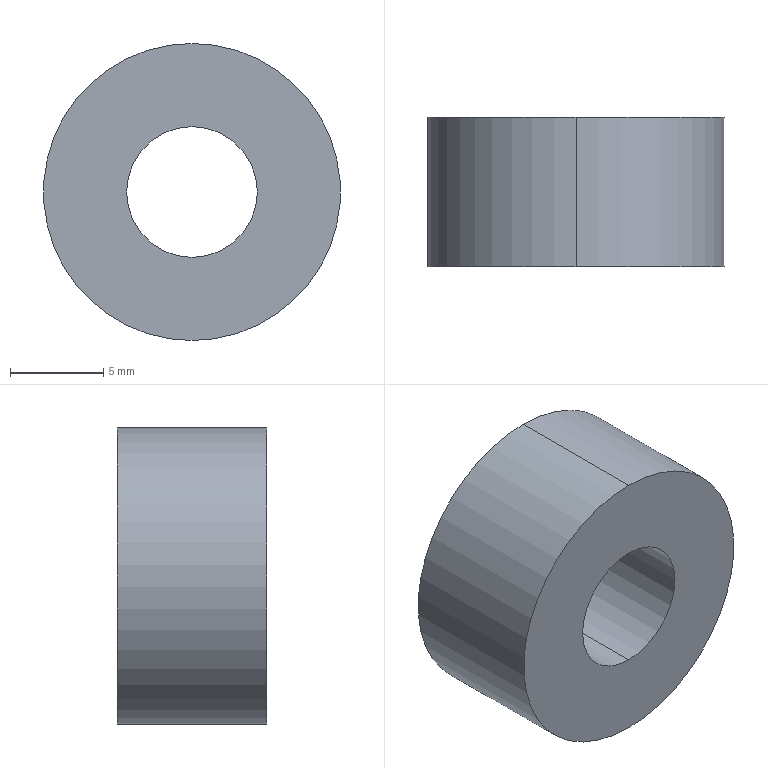Part | SolidWorks | features Extrusion 1 | 1 solid | 6 faces | box 15.9 x 8 x 15.9 mm | volume 1281 mm3 | cylinder 4 | plane 2 | commonest cylinder face diameters 7 x2 15.9 x2
STEP:
#1=CARTESIAN_POINT('',(0.,8.,-3.5));
#2=VERTEX_POINT('',#1);
#3=CARTESIAN_POINT('',(0.,8.,3.5));
#4=VERTEX_POINT('',#3);
#5=CARTESIAN_POINT('',(0.,8.,0.));
#6=DIRECTION('',(0.,1.,0.));
#7=DIRECTION('',(0.,0.,1.));
#8=AXIS2_PLACEMENT_3D('',#5,#6,#7);
#9=CIRCLE('',#8,3.5);
#10=EDGE_CURVE('',#2,#4,#9,.T.);
#11=ORIENTED_EDGE('',*,*,#10,.T.);
#12=CARTESIAN_POINT('',(0.,0.,3.5));
#13=VERTEX_POINT('',#12);
#14=CARTESIAN_POINT('',(0.,8.,3.5));
#15=DIRECTION('',(0.,-1.,0.));
#16=VECTOR('',#15,1000.);
#17=LINE('',#14,#16);
#18=EDGE_CURVE('',#4,#13,#17,.T.);
#19=ORIENTED_EDGE('',*,*,#18,.T.);
#20=CARTESIAN_POINT('',(0.,0.,-3.5));
#21=VERTEX_POINT('',#20);
#22=CARTESIAN_POINT('',(0.,0.,0.));
#23=DIRECTION('',(0.,1.,0.));
#24=DIRECTION('',(0.,0.,1.));
#25=AXIS2_PLACEMENT_3D('',#22,#23,#24);
#26=CIRCLE('',#25,3.5);
#27=EDGE_CURVE('',#21,#13,#26,.T.);
#28=ORIENTED_EDGE('',*,*,#27,.F.);
#29=CARTESIAN_POINT('',(0.,8.,-3.5));
#30=DIRECTION('',(0.,-1.,0.));
#31=VECTOR('',#30,1000.);
#32=LINE('',#29,#31);
#33=EDGE_CURVE('',#2,#21,#32,.T.);
#34=ORIENTED_EDGE('',*,*,#33,.F.);
#35=EDGE_LOOP('',(#11,#19,#28,#34));
#36=FACE_OUTER_BOUND('',#35,.T.);
#37=CARTESIAN_POINT('',(0.,8.,0.));
#38=DIRECTION('',(0.,-1.,0.));
#39=DIRECTION('',(0.,0.,-1.));
#40=AXIS2_PLACEMENT_3D('',#37,#38,#39);
#41=CYLINDRICAL_SURFACE('',#40,3.5);
#42=ADVANCED_FACE('',(#36),#41,.F.);
#43=CARTESIAN_POINT('',(0.,8.,7.95));
#44=VERTEX_POINT('',#43);
#45=CARTESIAN_POINT('',(0.,8.,-7.95));
#46=VERTEX_POINT('',#45);
#47=CARTESIAN_POINT('',(0.,8.,0.));
#48=DIRECTION('',(0.,1.,0.));
#49=DIRECTION('',(0.,0.,1.));
#50=AXIS2_PLACEMENT_3D('',#47,#48,#49);
#51=CIRCLE('',#50,7.95);
#52=EDGE_CURVE('',#44,#46,#51,.T.);
#53=ORIENTED_EDGE('',*,*,#52,.F.);
#54=CARTESIAN_POINT('',(0.,0.,7.95));
#55=VERTEX_POINT('',#54);
#56=CARTESIAN_POINT('',(0.,8.,7.95));
#57=DIRECTION('',(0.,-1.,0.));
#58=VECTOR('',#57,1000.);
#59=LINE('',#56,#58);
#60=EDGE_CURVE('',#44,#55,#59,.T.);
#61=ORIENTED_EDGE('',*,*,#60,.T.);
#62=CARTESIAN_POINT('',(0.,0.,-7.95));
#63=VERTEX_POINT('',#62);
#64=CARTESIAN_POINT('',(0.,0.,0.));
#65=DIRECTION('',(0.,1.,0.));
#66=DIRECTION('',(0.,0.,1.));
#67=AXIS2_PLACEMENT_3D('',#64,#65,#66);
#68=CIRCLE('',#67,7.95);
#69=EDGE_CURVE('',#55,#63,#68,.T.);
#70=ORIENTED_EDGE('',*,*,#69,.T.);
#71=CARTESIAN_POINT('',(0.,8.,-7.95));
#72=DIRECTION('',(0.,-1.,0.));
#73=VECTOR('',#72,1000.);
#74=LINE('',#71,#73);
#75=EDGE_CURVE('',#46,#63,#74,.T.);
#76=ORIENTED_EDGE('',*,*,#75,.F.);
#77=EDGE_LOOP('',(#53,#61,#70,#76));
#78=FACE_OUTER_BOUND('',#77,.T.);
#79=CARTESIAN_POINT('',(0.,8.,0.));
#80=DIRECTION('',(0.,-1.,0.));
#81=DIRECTION('',(0.,0.,-1.));
#82=AXIS2_PLACEMENT_3D('',#79,#80,#81);
#83=CYLINDRICAL_SURFACE('',#82,7.95);
#84=ADVANCED_FACE('',(#78),#83,.T.);
#85=CARTESIAN_POINT('',(0.,8.,0.));
#86=DIRECTION('',(0.,1.,0.));
#87=DIRECTION('',(0.,0.,1.));
#88=AXIS2_PLACEMENT_3D('',#85,#86,#87);
#89=CIRCLE('',#88,7.95);
#90=EDGE_CURVE('',#46,#44,#89,.T.);
#91=ORIENTED_EDGE('',*,*,#90,.T.);
#92=ORIENTED_EDGE('',*,*,#52,.T.);
#93=EDGE_LOOP('',(#91,#92));
#94=FACE_OUTER_BOUND('',#93,.T.);
#95=ORIENTED_EDGE('',*,*,#10,.F.);
#96=CARTESIAN_POINT('',(0.,8.,0.));
#97=DIRECTION('',(0.,1.,0.));
#98=DIRECTION('',(0.,0.,1.));
#99=AXIS2_PLACEMENT_3D('',#96,#97,#98);
#100=CIRCLE('',#99,3.5);
#101=EDGE_CURVE('',#4,#2,#100,.T.);
#102=ORIENTED_EDGE('',*,*,#101,.F.);
#103=EDGE_LOOP('',(#95,#102));
#104=FACE_BOUND('',#103,.T.);
#105=CARTESIAN_POINT('',(0.,8.,0.));
#106=DIRECTION('',(0.,1.,0.));
#107=DIRECTION('',(0.,0.,1.));
#108=AXIS2_PLACEMENT_3D('',#105,#106,#107);
#109=PLANE('',#108);
#110=ADVANCED_FACE('',(#94,#104),#109,.T.);
#111=CARTESIAN_POINT('',(0.,0.,0.));
#112=DIRECTION('',(0.,1.,0.));
#113=DIRECTION('',(0.,0.,1.));
#114=AXIS2_PLACEMENT_3D('',#111,#112,#113);
#115=CIRCLE('',#114,7.95);
#116=EDGE_CURVE('',#63,#55,#115,.T.);
#117=ORIENTED_EDGE('',*,*,#116,.F.);
#118=ORIENTED_EDGE('',*,*,#69,.F.);
#119=EDGE_LOOP('',(#117,#118));
#120=FACE_OUTER_BOUND('',#119,.T.);
#121=ORIENTED_EDGE('',*,*,#27,.T.);
#122=CARTESIAN_POINT('',(0.,0.,0.));
#123=DIRECTION('',(0.,1.,0.));
#124=DIRECTION('',(0.,0.,1.));
#125=AXIS2_PLACEMENT_3D('',#122,#123,#124);
#126=CIRCLE('',#125,3.5);
#127=EDGE_CURVE('',#13,#21,#126,.T.);
#128=ORIENTED_EDGE('',*,*,#127,.T.);
#129=EDGE_LOOP('',(#121,#128));
#130=FACE_BOUND('',#129,.T.);
#131=CARTESIAN_POINT('',(0.,0.,0.));
#132=DIRECTION('',(0.,1.,0.));
#133=DIRECTION('',(0.,0.,1.));
#134=AXIS2_PLACEMENT_3D('',#131,#132,#133);
#135=PLANE('',#134);
#136=ADVANCED_FACE('',(#120,#130),#135,.F.);
#137=ORIENTED_EDGE('',*,*,#60,.F.);
#138=ORIENTED_EDGE('',*,*,#90,.F.);
#139=ORIENTED_EDGE('',*,*,#75,.T.);
#140=ORIENTED_EDGE('',*,*,#116,.T.);
#141=EDGE_LOOP('',(#137,#138,#139,#140));
#142=FACE_OUTER_BOUND('',#141,.T.);
#143=CARTESIAN_POINT('',(0.,8.,0.));
#144=DIRECTION('',(0.,-1.,0.));
#145=DIRECTION('',(0.,0.,-1.));
#146=AXIS2_PLACEMENT_3D('',#143,#144,#145);
#147=CYLINDRICAL_SURFACE('',#146,7.95);
#148=ADVANCED_FACE('',(#142),#147,.T.);
#149=ORIENTED_EDGE('',*,*,#18,.F.);
#150=ORIENTED_EDGE('',*,*,#101,.T.);
#151=ORIENTED_EDGE('',*,*,#33,.T.);
#152=ORIENTED_EDGE('',*,*,#127,.F.);
#153=EDGE_LOOP('',(#149,#150,#151,#152));
#154=FACE_OUTER_BOUND('',#153,.T.);
#155=CARTESIAN_POINT('',(0.,8.,0.));
#156=DIRECTION('',(0.,-1.,0.));
#157=DIRECTION('',(0.,0.,-1.));
#158=AXIS2_PLACEMENT_3D('',#155,#156,#157);
#159=CYLINDRICAL_SURFACE('',#158,3.5);
#160=ADVANCED_FACE('',(#154),#159,.F.);
#161=CLOSED_SHELL('',(#42,#84,#110,#136,#148,#160));
#162=MANIFOLD_SOLID_BREP('',#161);
#163=CARTESIAN_POINT('',(0.,0.,0.));
#164=DIRECTION('',(0.,0.,1.));
#165=DIRECTION('',(1.,0.,0.));
#166=AXIS2_PLACEMENT_3D('',#163,#164,#165);
#167=(LENGTH_UNIT()NAMED_UNIT(*)SI_UNIT(.MILLI.,.METRE.));
#168=UNCERTAINTY_MEASURE_WITH_UNIT(LENGTH_MEASURE(0.00001),#167,'','');
#169=(NAMED_UNIT(*)PLANE_ANGLE_UNIT()SI_UNIT($,.RADIAN.));
#170=(NAMED_UNIT(*)SI_UNIT($,.STERADIAN.)SOLID_ANGLE_UNIT());
#171=(GEOMETRIC_REPRESENTATION_CONTEXT(3)GLOBAL_UNCERTAINTY_ASSIGNED_CONTEXT((#168))GLOBAL_UNIT_ASSIGNED_CONTEXT((#167,#169,#170))REPRESENTATION_CONTEXT('',''));
#172=ADVANCED_BREP_SHAPE_REPRESENTATION('',(#162,#166),#171);